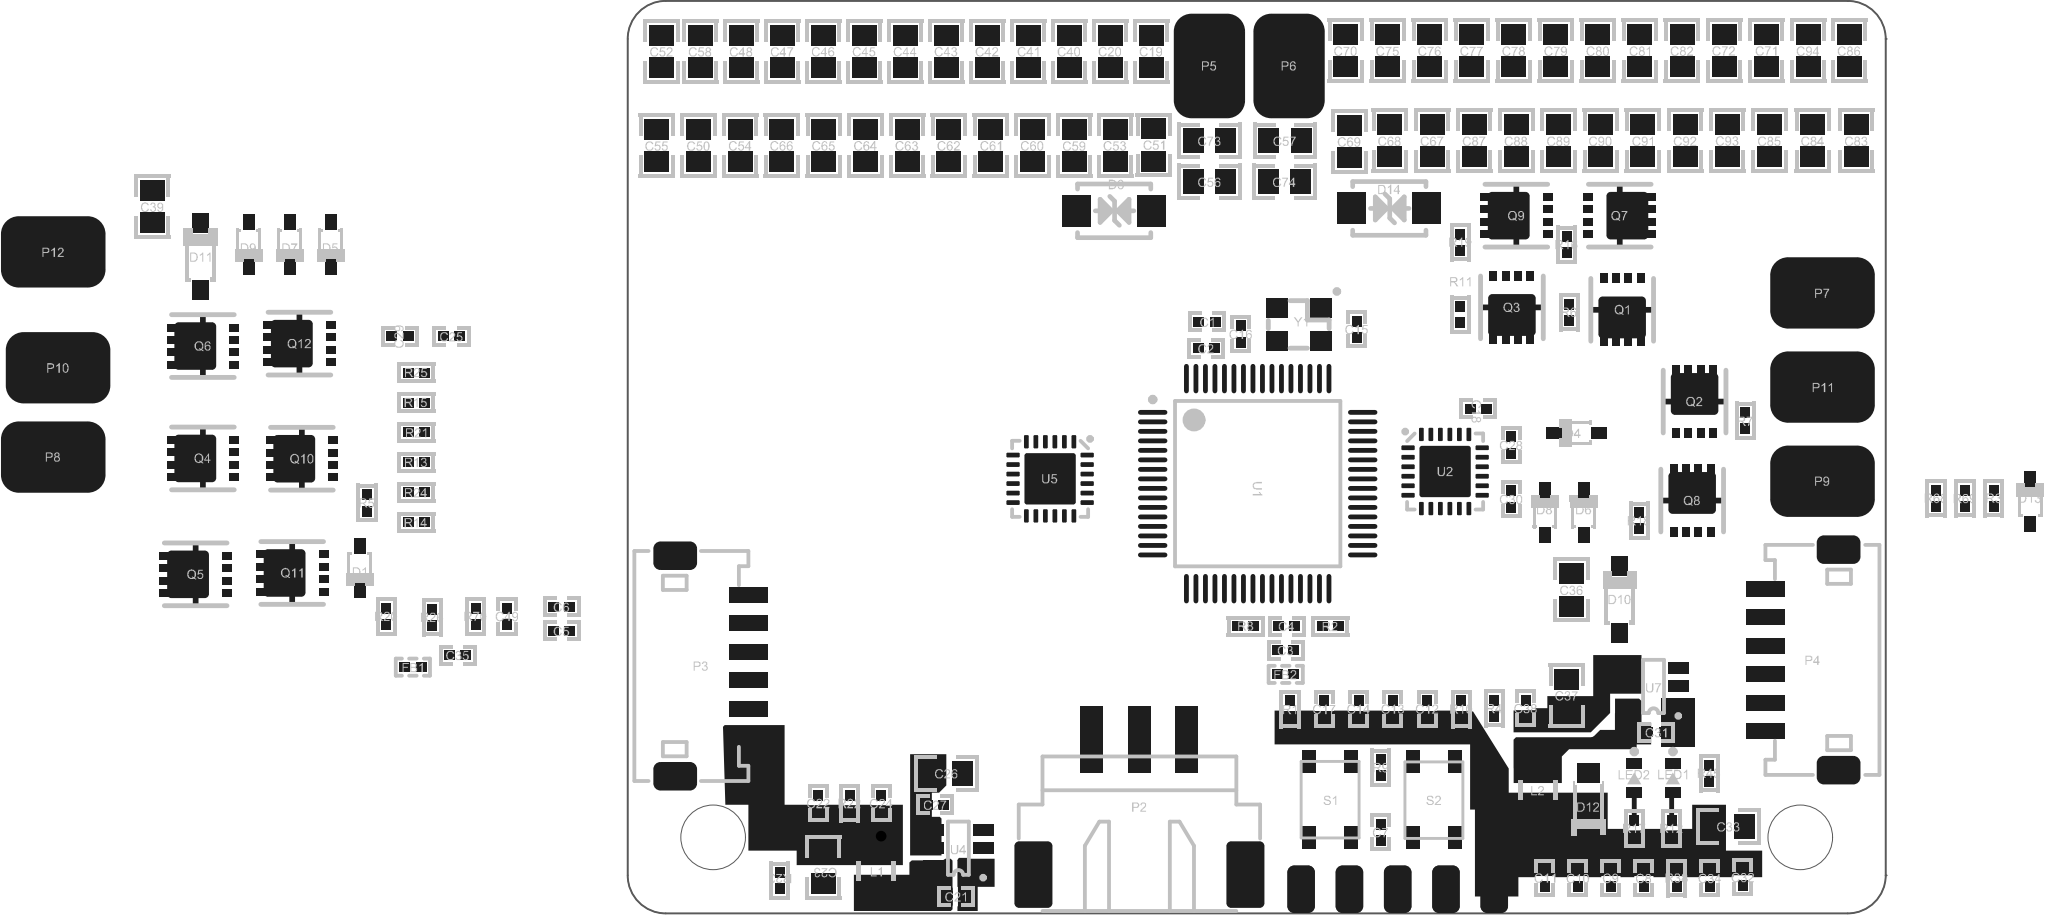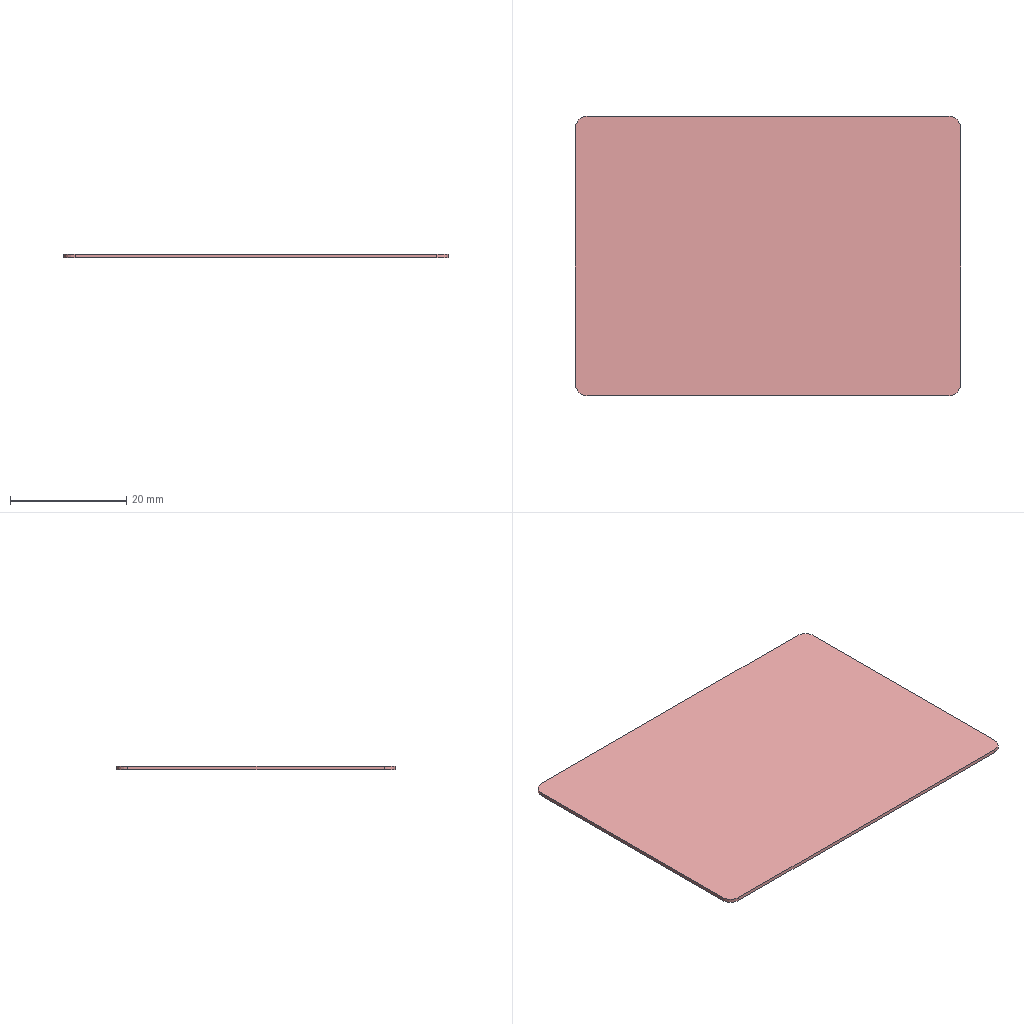Circuit board layout | Altium Designer | box 66.2 x 48 x 0.6 mm
Layer stack:
# Altium Designer layer stack of  (unit mm; dielectric type: 0 none, 1 core, 2 prepreg, 3 surface material)
index,name,kind,layer,copper_thickness_mm,dielectric_type,dielectric_thickness_mm,dielectric_material,dielectric_constant
0,Top Solder Mask Layer,dielectric,,,3,0.0102,Solder Resist,3.5
1,Top Layer,copper,Top Layer,0.0356,,,,
2,Dielectric 3,dielectric,,,3,0.0711,PP-006,4.1
3,GND,copper,GND,0.035,,,,
4,Dielectric 2,dielectric,,,3,0.0711,PP-006,4.1
5,POWER,copper,POWER,0.035,,,,
6,Dielectric 1,dielectric,,,3,0.32,FR-4,4.8
7,Bottom Layer,copper,Bottom Layer,0.0356,,,,
8,Bottom Solder Mask Layer,dielectric,,,3,0.0102,Solder Resist,3.5
# drill layer pairs: low layer,high layer
drill_pair,Top Layer,Bottom Layer
Part placement:
Designator,Comment,Layer,Footprint,Center-X(mm),Center-Y(mm),Rotation
Y1,16MHz 20pF,TopLayer,X3225-4,144.482,110.296,180
U5,FD6288Q,TopLayer,QFN24-4x4-L,131.401,102.168,270
U7,RY9121E,TopLayer,SOT-23-6,163.151,91.246,180
U4,RY9121E,TopLayer,SOT-23-6,126.575,82.737,180
U2,FD6288Q,TopLayer,QFN24-4x4-L,152.184,102.553,0
U1,CYT2BL3CAx,TopLayer,LQFP64_L,142.323,101.914,0
S2,KEY-TS1145,TopLayer,TS1145-B-A,151.594,85.277,90
S1,KEY-TS1145,TopLayer,TS1145-B-A,146.133,85.277,270
R70,100R ±1%,TopLayer,RESC1005[0402]S-N,101.175,94.929,90
R69,10K ±1%,TopLayer,RESC1005[0402]S-N,179.534,101.152,270
R68,1K ±1%,TopLayer,RESC1005[0402]S-N,178.01,101.152,90
R45,10K ±1%,TopLayer,RESC1005[0402]S-N,166.072,86.674,90
R38,45.3K ±1%,TopLayer,RESC1005[0402]S-N,164.38,81.169,90
R26,100R ±1%,TopLayer,RESC1005[0402]S-N,98.889,94.885,270
R25,4.7R ±1%,TopLayer,RESC1005[0402]S-N,98.044,107.756,180
R24,4.7R ±1%,TopLayer,RESC1005[0402]S-N,98.044,101.457,180
R23,10K ±1%,TopLayer,RESC1005[0402]S-N,117.177,81.022,270
R22,73.2K ±1%,TopLayer,RESC1005[0402]S-N,120.86,85.106,270
R21,4.7R ±1%,TopLayer,RESC1005[0402]S-N,98.044,104.607,180
R20,100R ±1%,TopLayer,RESC1005[0402]S-N,96.476,94.929,270
R19,4.7R ±1%,TopLayer,RESC1005[0402]S-N,152.991,114.614,90
R18,4.7R ±1%,TopLayer,RESC1005[0402]S-N,162.389,99.965,270
R17,1K ±1%,TopLayer,RESC1005[0402]S-N,162.135,83.777,90
R16,4.7R ±1%,TopLayer,RESC1005[0402]S-N,158.579,114.487,90
R15,4.7R ±1%,TopLayer,RESC1005[0402]S-N,98.044,106.181,180
R14,4.7R ±1%,TopLayer,RESC1005[0402]S-N,98.044,99.882,180
R13,4.7R ±1%,TopLayer,RESC1005[0402]S-N,98.044,103.032,180
R12,1K ±1%,TopLayer,RESC1005[0402]S-N,164.104,83.777,90
R11,4.7R ±1%,TopLayer,RESC1005[0402]S-N,152.991,110.804,90
R10,4.7K ±1%,TopLayer,RESC1005[0402]S-N,153.042,90.058,90
R9,100R ±1%,TopLayer,RESC1005[0402]S-N,148.8,86.972,270
R8,0R ±1%,TopLayer,RESC1005[0402]S-N,141.688,94.421,180
R7,4.7R ±1%,TopLayer,RESC1005[0402]S-N,167.977,105.216,270
R6,4.7R ±1%,TopLayer,RESC1005[0402]S-N,158.706,110.931,90
R5,100R ±1%,TopLayer,RESC1005[0402]S-N,95.46,100.898,270
R4,100R ±1%,TopLayer,RESC1005[0402]S-N,154.769,90.103,270
R3,100R ±1%,TopLayer,RESC1005[0402]S-N,181.058,101.152,90
R2,0R ±1%,TopLayer,RESC1005[0402]S-N,146.133,94.421,0
R1,10K ±1%,TopLayer,RESC1005[0402]S-N,144.025,90.058,90
Q12,TPN2R703NL,TopLayer,TSON3x3,91.904,109.28,90
Q11,TPN2R703NL,TopLayer,TSON3x3,91.523,97.215,90
Q10,TPN2R703NL,TopLayer,TSON3x3,92.032,103.225,90
Q9,TPN2R703NL,TopLayer,TSON3x3,155.931,116.011,90
Q8,TPN2R703NL,TopLayer,TSON3x3,165.183,101.025,0
Q7,TPN2R703NL,TopLayer,TSON3x3,161.373,116.011,270
Q6,TPN2R703NL,TopLayer,TSON3x3,86.824,109.153,90
Q5,TPN2R703NL,TopLayer,TSON3x3,86.444,97.144,90
Q4,TPN2R703NL,TopLayer,TSON3x3,86.825,103.24,90
Q3,TPN2R703NL,TopLayer,TSON3x3,155.699,111.186,180
Q2,TPN2R703NL,TopLayer,TSON3x3,165.31,106.232,0
Q1,TPN2R703NL,TopLayer,TSON3x3,161.5,111.058,180
P12,WirePad,TopLayer,WirePad-4x6,78.95,114.106,0
P11,WirePad,TopLayer,WirePad-4x6,172.041,106.994,0
P10,WirePad,TopLayer,WirePad-4x6,79.204,108.01,0
P9,WirePad,TopLayer,WirePad-4x6,172.041,102.041,0
P8,WirePad,TopLayer,WirePad-4x6,78.95,103.311,0
P7,WirePad,TopLayer,WirePad-4x6,172.041,111.947,0
P6,WirePad,TopLayer,WirePad-4x6,143.974,123.885,90
P5,WirePad,TopLayer,WirePad-4x6,139.783,123.885,90
P4,ZH1.5-6P,TopLayer,ZH1.5-6P-SH,170.962,92.643,90
P3,ZH1.5-6P,TopLayer,ZH1.5-6P-SH,113.601,92.322,270
P2,XH2.54-3P,TopLayer,XH2.54-3P-SH,136.1,84.915,0
P1,SWD Header 5x2,BottomLayer,HDR2X5-OB,149.689,80.578,270
LED2,Blue SMD LED,TopLayer,LEDC1608(0603)-L,162.135,86.42,270
LED1,Red SMD LED,TopLayer,LEDC1608(0603)-L,164.167,86.42,270
L2,4.7uH 2A,TopLayer,SLO2520,157.055,85.785,90
L1,4.7uH 2A,TopLayer,SLO2520,122.257,81.523,270
FB2,120R @100MHz 500mA,TopLayer,INDC1005[0402]S,143.798,91.881,180
FB1,120R @100MHz 500mA,TopLayer,INDC1005[0402]S,97.873,92.262,0
D14,SMAJ16CA,TopLayer,SMA[DO-214AC]-Bi,149.249,116.392,180
D13,B5819WS,TopLayer,SOD-323,182.963,100.993,90
D12,SMF3.3A,TopLayer,SOD-123-FL,159.722,84.924,270
D11,BZT52C15,TopLayer,SOD-123-L,86.697,113.852,90
D10,BZT52C15,TopLayer,SOD-123-L,161.373,95.818,90
D9,B5819WS,TopLayer,SOD-323,89.237,114.487,270
D8,B5819WS,TopLayer,SOD-323,157.436,100.39,90
D7,B5819WS,TopLayer,SOD-323,91.396,114.487,270
D6,B5819WS,TopLayer,SOD-323,159.468,100.39,90
D5,B5819WS,TopLayer,SOD-323,93.555,114.487,270
D4,B5819WS,TopLayer,SOD-323,159.087,104.581,180
D3,SMAJ16CA,TopLayer,SMA[DO-214AC]-Bi,134.77,116.265,180
D1,B5819WS,TopLayer,SOD-323,95.079,97.469,270
C94,22uF 25V X5R,TopLayer,CAPC2012[0805]S-N,171.279,124.686,270
C93,22uF 25V X5R,TopLayer,CAPC2012[0805]S-N,167.028,119.948,90
C92,22uF 25V X5R,TopLayer,CAPC2012[0805]S-N,164.81,119.948,90
C91,22uF 25V X5R,TopLayer,CAPC2012[0805]S-N,162.591,119.948,90
C90,22uF 25V X5R,TopLayer,CAPC2012[0805]S-N,160.372,119.948,90
C89,22uF 25V X5R,TopLayer,CAPC2012[0805]S-N,158.154,119.948,90
C88,22uF 25V X5R,TopLayer,CAPC2012[0805]S-N,155.935,119.948,90
C87,22uF 25V X5R,TopLayer,CAPC2012[0805]S-N,153.716,119.948,90
C86,22uF 25V X5R,TopLayer,CAPC2012[0805]S-N,173.438,124.686,270
C85,22uF 25V X5R,TopLayer,CAPC2012[0805]S-N,169.247,119.949,90
C84,22uF 25V X5R,TopLayer,CAPC2012[0805]S-N,171.533,119.948,90
C83,22uF 25V X5R,TopLayer,CAPC2012[0805]S-N,173.819,119.948,90
C82,22uF 25V X5R,TopLayer,CAPC2012[0805]S-N,164.648,124.686,270
C81,22uF 25V X5R,TopLayer,CAPC2012[0805]S-N,162.437,124.686,270
C80,22uF 25V X5R,TopLayer,CAPC2012[0805]S-N,160.227,124.686,270
C79,22uF 25V X5R,TopLayer,CAPC2012[0805]S-N,158.016,124.686,270
C78,22uF 25V X5R,TopLayer,CAPC2012[0805]S-N,155.805,124.686,270
C77,22uF 25V X5R,TopLayer,CAPC2012[0805]S-N,153.595,124.686,270
C76,22uF 25V X5R,TopLayer,CAPC2012[0805]S-N,151.385,124.686,270
C75,22uF 25V X5R,TopLayer,CAPC2012[0805]S-N,149.174,124.686,270
C74,22uF 25V X5R,TopLayer,CAPC2012[0805]S-N,143.72,117.789,0
C73,22uF 25V X5R,TopLayer,CAPC2012[0805]S-N,139.783,119.948,180
C72,22uF 25V X5R,TopLayer,CAPC2012[0805]S-N,166.858,124.686,270
C71,22uF 25V X5R,TopLayer,CAPC2012[0805]S-N,169.069,124.686,270
C70,22uF 25V X5R,TopLayer,CAPC2012[0805]S-N,146.964,124.686,270
C69,22uF 25V X5R,TopLayer,CAPC2012[0805]S-N,147.149,119.909,90
C68,22uF 25V X5R,TopLayer,CAPC2012[0805]S-N,149.279,119.948,90
C67,22uF 25V X5R,TopLayer,CAPC2012[0805]S-N,151.498,119.949,90
C66,22uF 25V X5R,TopLayer,CAPC2012[0805]S-N,117.291,119.694,270
C65,22uF 25V X5R,TopLayer,CAPC2012[0805]S-N,119.489,119.694,270
C64,22uF 25V X5R,TopLayer,CAPC2012[0805]S-N,121.685,119.694,270
C63,22uF 25V X5R,TopLayer,CAPC2012[0805]S-N,123.883,119.694,270
C62,22uF 25V X5R,TopLayer,CAPC2012[0805]S-N,126.08,119.694,270
C61,22uF 25V X5R,TopLayer,CAPC2012[0805]S-N,128.277,119.694,270
C60,22uF 25V X5R,TopLayer,CAPC2012[0805]S-N,130.474,119.694,270
C59,22uF 25V X5R,TopLayer,CAPC2012[0805]S-N,132.671,119.694,270
C58,22uF 25V X5R,TopLayer,CAPC2012[0805]S-N,112.986,124.647,90
C57,22uF 25V X5R,TopLayer,CAPC2012[0805]S-N,143.759,119.948,180
C56,22uF 25V X5R,TopLayer,CAPC2012[0805]S-N,139.783,117.789,0
C55,22uF 25V X5R,TopLayer,CAPC2012[0805]S-N,110.7,119.694,270
C54,22uF 25V X5R,TopLayer,CAPC2012[0805]S-N,115.094,119.694,270
C53,22uF 25V X5R,TopLayer,CAPC2012[0805]S-N,134.83,119.694,270
C52,22uF 25V X5R,TopLayer,CAPC2012[0805]S-N,110.954,124.647,90
C51,22uF 25V X5R,TopLayer,CAPC2012[0805]S-N,136.862,119.733,270
C50,22uF 25V X5R,TopLayer,CAPC2012[0805]S-N,112.897,119.694,270
C49,100nF 16V X7R,TopLayer,CAPC1005[0402]S-N,102.826,94.929,270
C48,22uF 25V X5R,TopLayer,CAPC2012[0805]S-N,115.145,124.647,90
C47,22uF 25V X5R,TopLayer,CAPC2012[0805]S-N,117.302,124.647,90
C46,22uF 25V X5R,TopLayer,CAPC2012[0805]S-N,119.459,124.647,90
C45,22uF 25V X5R,TopLayer,CAPC2012[0805]S-N,121.616,124.647,90
C44,22uF 25V X5R,TopLayer,CAPC2012[0805]S-N,123.773,124.647,90
C43,22uF 25V X5R,TopLayer,CAPC2012[0805]S-N,125.929,124.647,90
C42,22uF 25V X5R,TopLayer,CAPC2012[0805]S-N,128.086,124.647,90
C41,22uF 25V X5R,TopLayer,CAPC2012[0805]S-N,130.243,124.647,90
C40,22uF 25V X5R,TopLayer,CAPC2012[0805]S-N,132.4,124.647,90
C39,22uF 25V X5R,TopLayer,CAPC2012[0805]S-N,84.157,116.48,90
C38,100nF 16V X7R,TopLayer,CAPC1005[0402]S-N,156.42,90.103,270
C37,22uF 25V X5R,TopLayer,CAPC2012[0805]S-N,158.579,90.777,270
C36,22uF 25V X5R,TopLayer,CAPC2012[0805]S-N,158.833,96.326,270
C35,4.7uF 10V X5R,TopLayer,CAPC1005[0402]S-N,100.242,92.897,0
C34,100nF 16V X7R,TopLayer,CAPC1005[0402]S-N,166.114,81.169,90
C33,22uF 25V X5R,TopLayer,CAPC2012[0805]S-N,167.088,83.88,180
C32,220pF 50V X7R,TopLayer,CAPC1005[0402]S-N,167.85,81.213,90
C31,100nF 16V X7R,TopLayer,CAPC1005[0402]S-N,163.278,88.833,180
C30,4.7uF 10V X5R,TopLayer,CAPC1005[0402]S-N,155.658,101.108,90
C29,4.7uF 10V X5R,TopLayer,CAPC1005[0402]S-N,97.194,109.661,0
C28,4.7uF 10V X5R,TopLayer,CAPC1005[0402]S-N,155.658,103.946,270
C27,100nF 16V X7R,TopLayer,CAPC1005[0402]S-N,125.349,85.023,180
C26,22uF 25V X5R,TopLayer,CAPC2012[0805]S-N,125.94,86.674,180
C25,4.7uF 10V X5R,TopLayer,CAPC1005[0402]S-N,99.905,109.661,0
C24,100nF 16V X7R,TopLayer,CAPC1005[0402]S-N,122.511,85.106,270
C23,22uF 25V X5R,TopLayer,CAPC2012[0805]S-N,119.463,81.721,90
C22,220pF 50V X7R,TopLayer,CAPC1005[0402]S-N,119.209,85.106,270
C21,100nF 16V X7R,TopLayer,CAPC1005[0402]S-N,126.448,80.197,180
C20,22uF 25V X5R,TopLayer,CAPC2012[0805]S-N,134.557,124.647,90
C19,22uF 25V X5R,TopLayer,CAPC2012[0805]S-N,136.714,124.647,90
C18,4.7uF 10V X5R,TopLayer,CAPC1005[0402]S-N,153.924,105.851,180
C17,100nF 16V X7R,TopLayer,CAPC1005[0402]S-N,145.828,90.059,270
C16,10pF 50V C0G,TopLayer,CAPC1005[0402]S-N,141.434,109.788,270
C15,10pF 50V C0G,TopLayer,CAPC1005[0402]S-N,147.53,110.042,270
C14,4.7uF 10V X5R,TopLayer,CAPC1005[0402]S-N,147.632,90.059,270
C13,100nF 16V X7R,TopLayer,CAPC1005[0402]S-N,149.435,90.059,270
C12,4.7uF 10V X5R,TopLayer,CAPC1005[0402]S-N,151.238,90.059,270
C11,100nF 16V X7R,TopLayer,CAPC1005[0402]S-N,157.436,81.171,270
C10,100nF 16V X7R,TopLayer,CAPC1005[0402]S-N,159.171,81.169,90
C9,4.7uF 10V X5R,TopLayer,CAPC1005[0402]S-N,160.907,81.17,270
C8,4.7uF 10V X5R,TopLayer,CAPC1005[0402]S-N,162.643,81.169,90
C7,100nF 16V X7R,TopLayer,CAPC1005[0402]S-N,148.8,83.582,270
C6,100nF 16V X7R,TopLayer,CAPC1005[0402]S-N,105.703,95.437,0
C5,2.2uF 10V X5R,TopLayer,CAPC1005[0402]S-N,105.703,94.167,0
C4,100nF 16V X7R,TopLayer,CAPC1005[0402]S-N,143.847,94.421,0
C3,4.7uF 10V X5R,TopLayer,CAPC1005[0402]S-N,143.803,93.151,180
C2,100nF 16V X7R,TopLayer,CAPC1005[0402]S-N,139.612,109.026,0
C1,4.7uF 10V X5R,TopLayer,CAPC1005[0402]S-N,139.656,110.423,0
Pad and via stacks:
# Altium Designer via and pad stacks of  (unit mm). Each distinct definition once, with the count of objects using it.
# via: kind,start_layer,end_layer,hole_mm,diameter_mm,mode(0 simple;1 top-mid-bottom;2 full stack),diameter_per_layer,count,example_net
# pad: kind,layer,hole_mm,hole_type(0 round;1 square;2 slot),plating,top_size,top_shape(1 round;2 rect;3 octagon;9 rounded rect),mid_size,bottom_size,mode,footprint,size_per_layer,count,example
pad,Top Layer,0,0,plated,1.143x1,2,1.143x1,1.143x1,0,X3225-4,,4,Y1.2
pad,Top Layer,0,0,plated,0.7x0.25,9,0.7x0.25,0.7x0.25,0,QFN24-4x4-L,,48,U5.24
pad,Top Layer,0,0,plated,2.7x2.7,9,2.7x2.7,2.7x2.7,0,QFN24-4x4-L,,2,U5.25
pad,Top Layer,0,0,plated,0.6x1.1,2,0.6x1.1,0.6x1.1,0,SOT-23-6,,12,U7.1
pad,Top Layer,0,0,plated,0.254x1.55,1,0.254x1.55,0.254x1.55,0,LQFP64_L,,64,U1.1
pad,Top Layer,0,0,plated,0.7x1.2,2,0.7x1.2,0.7x1.2,0,TS1145-B-A,,8,S2.1
pad,Top Layer,0,0,plated,0.5x0.55,2,0.5x0.55,0.5x0.55,0,RESC1005[0402]S-N,,62,R70.1
pad,Top Layer,0,0,plated,2.5x2.2,9,2.5x2.2,2.5x2.2,0,TSON3x3,,12,Q12.1
pad,Top Layer,0,0,plated,0.4x0.5,2,0.4x0.5,0.4x0.5,0,TSON3x3,,96,Q12.2
pad,Top Layer,0,0,plated,3.4x0.3,9,3.4x0.3,3.4x0.3,0,TSON3x3,,12,Q12.1
pad,Top Layer,0,0,plated,5.5x3.75,9,5.5x3.75,5.5x3.75,0,WirePad-4x6,,8,P12.1
pad,Top Layer,0,0,plated,1.5x2.3,9,1.5x2.3,1.5x2.3,0,ZH1.5-6P-SH,,4,P4.0
pad,Top Layer,0,0,plated,0.8x2,2,0.8x2,0.8x2,0,ZH1.5-6P-SH,,12,P4.6
pad,Top Layer,0,0,plated,2x3.5,9,2x3.5,2x3.5,0,XH2.54-3P-SH,,2,P2.0
pad,Top Layer,0,0,plated,1.2x3.5,2,1.2x3.5,1.2x3.5,0,XH2.54-3P-SH,,3,P2.1
pad,Top Layer,0,0,plated,2.5x1.45,9,2.5x1.45,2.5x1.45,0,HDR2X5-OB,,5,P1.4
pad,Top Layer,0,0,unplated,0.55x0.8,2,0.55x0.8,0.55x0.8,0,LEDC1608(0603)-L,,4,LED2.C
pad,Top Layer,0,0,plated,0.8x2,2,0.8x2,0.8x2,0,SLO2520,,4,L2.2
pad,Top Layer,0,0,plated,0.5x0.55,2,0.5x0.55,0.5x0.55,0,INDC1005[0402]S,,4,FB2.2
pad,Top Layer,0,0,unplated,1.52x1.68,2,1.52x1.68,1.52x1.68,0,SMA[DO-214AC]-Bi,,4,D14.A
pad,Top Layer,0,0,unplated,0.8x0.6,2,0.8x0.6,0.8x0.6,0,SOD-323,,16,D13.A
pad,Top Layer,0,0,unplated,1x1.2,2,1x1.2,1x1.2,0,SOD-123-FL,,2,D12.K
pad,Top Layer,0,0,unplated,1x0.85,2,1x0.85,1x0.85,0,SOD-123-L,,4,D11.K
pad,Top Layer,0,0,plated,1.3x1.1,2,1.3x1.1,1.3x1.1,0,CAPC2012[0805]S-N,,124,C94.2
pad,Top Layer,0,0,plated,0.5x0.55,2,0.5x0.55,0.5x0.55,0,CAPC1005[0402]S-N,,64,C49.2
pad,Bottom Layer,0,0,plated,2.5x1.45,9,2.5x1.45,2.5x1.45,0,HDR2X5-OB,,5,P1.1
via,Top Layer,Bottom Layer,0.3048,0.5588,0,,1,VCC5V
Copper pours:
name,layer,net,type(0 solid;1 hatched;2 none)
Top Layer-NETC26_2,Top Layer,NETC26_2,0
Top Layer-VCC5V,Top Layer,VCC5V,0
Top Layer-NETC31_1,Top Layer,NETC31_1,0
Top Layer-NETC31_2,Top Layer,NETC31_2,0
Top Layer-NETC31_2 1,Top Layer,NETC31_2,0
Top Layer-NETC37_2,Top Layer,NETC37_2,0
Top Layer-NETC21_1,Top Layer,NETC21_1,0
Top Layer-NETC21_2,Top Layer,NETC21_2,0
Top Layer-VCC3V3,Top Layer,VCC3V3,0
Top Layer-VCC3V3 1,Top Layer,VCC3V3,0
Design rules, without the lines most boards share:
# Altium Designer design rules of  (exported by Altium Designer, unit mm)
# columns: name | kind | enabled | priority | scope1 | scope2 | descriptor | typed fields (field=value)
DiffPairsRouting_1 | 51 | enabled | 1 | All | All | Differential Pairs Uncoupled Length using the Gap Constraints (Min=10mil) (Max=10mil) (Prefered=10mil)  and Width Constraints (Min=15mil) (Max=15mil) (Prefered=15mil) (All) |
SolderMaskExpansion_1 | 13 | enabled | 1 | All | All | Solder Mask Expansion (Expansion =4mil) (All) | expansion=0.1016
PasteMaskExpansion_1 | 14 | enabled | 1 | All | All | Paste Mask Expansion (Expansion =0mil) (All) | expansion=0
RoutingVias_1 | 11 | enabled | 1 | All | All | Routing Via (MinHoleWidth=28mil) (MaxHoleWidth=28mil) (PreferredHoleWidth=28mil) (MinWidth=50mil) (MaxWidth=50mil) (PreferedWidth=50mil) (All) | via_min_hole=0.7112 via_max_hole=0.7112 via_preferred_diameter=1.27 via_preferred_hole=0.7112
Width_1 | 2 | enabled | 1 | All | All | Width Constraint (Min=10mil) (Max=10mil) (Preferred=10mil) (All) |
PolygonConnect_1 | 20 | enabled | 1 | All | All | Polygon Connect Rule(Relief Connect )(Conductor Width=10mil) (Relief Angle=90 Angle) (Entries=4) (Air Gap Width=10mil) (All),(All) | connect_style(0=relief,1=direct,2=none)=0 relief_conductor_width=0.254 relief_entries=4
PlaneConnect_1 | 6 | enabled | 1 | All | All | Power Plane Connect Rule(Relief Connect )(Expansion=20mil) (Conductor Width=10mil) (Air Gap=10mil) (Entries=4) (All) | relief_conductor_width=0.254 relief_entries=4 relief_expansion=0.508
Clearance_2 | 0 | enabled | 1 | All | All | Clearance Constraint (Gap=10mil) (All),(All) | gap=0.254
Clearance_1 | 52 | disabled | 1 | All | All | Hole To Hole Clearance (Gap=11.8mil) (Disabled)(All),(All) | gap=0.2997
Clearance | 52 | disabled | 2 | All | All | Hole To Hole Clearance (Gap=11.8mil) (Disabled)(All),(All) | gap=0.2997
Width | 52 | disabled | 3 | All | All | Hole To Hole Clearance (Gap=120mil) (Disabled)(All),(All) | gap=3.048
DiffPairsRouting | 52 | disabled | 4 | All | All | Hole To Hole Clearance (Gap=15mil) (Disabled)(All),(All) | gap=0.381
RoutingVias | 52 | disabled | 5 | All | All | Hole To Hole Clearance (Gap=25mil) (Disabled)(All),(All) | gap=0.635
PlaneConnect | 52 | disabled | 6 | All | All | Hole To Hole Clearance (Gap=1mil) (Disabled)(All),(All) | gap=0.0254
PolygonConnect | 52 | disabled | 7 | All | All | Hole To Hole Clearance (Gap=1mil) (Disabled)(All),(All) | gap=0.0254
SolderMaskExpansion | 52 | disabled | 8 | All | All | Hole To Hole Clearance (Gap=4mil) (Disabled)(All),(All) | gap=0.1016
PasteMaskExpansion | 52 | disabled | 9 | All | All | Hole To Hole Clearance (Gap=11.8mil) (Disabled)(All),(All) | gap=0.2997
HoleToHoleClearance | 52 | enabled | 10 | All | All | Hole To Hole Clearance (Gap=10mil) (All),(All) | gap=0.254